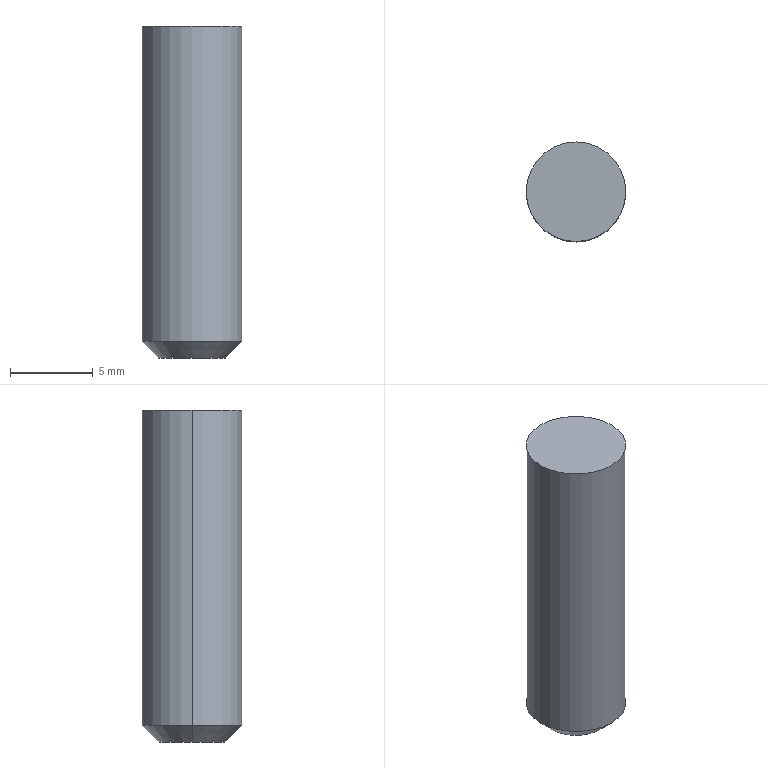Part | SolidWorks | features BaseBody 1 | 1 solid | 6 faces | box 6 x 6 x 20 mm | volume 557.109 mm3 | cylinder 2 | cone 2 | plane 2 | commonest cylinder face diameters 6 x2
STEP:
#1=CARTESIAN_POINT('',(403.071,348.177,19.477));
#2=VERTEX_POINT('',#1);
#3=CARTESIAN_POINT('',(409.071,348.177,19.477));
#4=VERTEX_POINT('',#3);
#5=CARTESIAN_POINT('',(406.071,348.177,19.477));
#6=DIRECTION('',(0.,0.,-1.));
#7=DIRECTION('',(-1.,0.,0.));
#8=AXIS2_PLACEMENT_3D('',#5,#6,#7);
#9=CIRCLE('',#8,3.);
#10=EDGE_CURVE('',#2,#4,#9,.T.);
#11=ORIENTED_EDGE('',*,*,#10,.F.);
#12=CARTESIAN_POINT('',(403.071,348.177,38.477));
#13=VERTEX_POINT('',#12);
#14=CARTESIAN_POINT('',(403.071,348.177,18.477));
#15=DIRECTION('',(0.,0.,1.));
#16=VECTOR('',#15,1000.);
#17=LINE('',#14,#16);
#18=EDGE_CURVE('',#2,#13,#17,.T.);
#19=ORIENTED_EDGE('',*,*,#18,.T.);
#20=CARTESIAN_POINT('',(409.071,348.177,38.477));
#21=VERTEX_POINT('',#20);
#22=CARTESIAN_POINT('',(406.071,348.177,38.477));
#23=DIRECTION('',(0.,0.,1.));
#24=DIRECTION('',(-1.,0.,0.));
#25=AXIS2_PLACEMENT_3D('',#22,#23,#24);
#26=CIRCLE('',#25,3.);
#27=EDGE_CURVE('',#21,#13,#26,.T.);
#28=ORIENTED_EDGE('',*,*,#27,.F.);
#29=CARTESIAN_POINT('',(409.071,348.177,18.477));
#30=DIRECTION('',(0.,0.,1.));
#31=VECTOR('',#30,1000.);
#32=LINE('',#29,#31);
#33=EDGE_CURVE('',#4,#21,#32,.T.);
#34=ORIENTED_EDGE('',*,*,#33,.F.);
#35=EDGE_LOOP('',(#11,#19,#28,#34));
#36=FACE_OUTER_BOUND('',#35,.T.);
#37=CARTESIAN_POINT('',(406.071,348.177,18.477));
#38=DIRECTION('',(0.,0.,1.));
#39=DIRECTION('',(1.,0.,0.));
#40=AXIS2_PLACEMENT_3D('',#37,#38,#39);
#41=CYLINDRICAL_SURFACE('',#40,3.);
#42=ADVANCED_FACE('',(#36),#41,.T.);
#43=CARTESIAN_POINT('',(404.071,348.177,18.477));
#44=VERTEX_POINT('',#43);
#45=CARTESIAN_POINT('',(408.071,348.177,18.477));
#46=VERTEX_POINT('',#45);
#47=CARTESIAN_POINT('',(406.071,348.177,18.477));
#48=DIRECTION('',(0.,0.,-1.));
#49=DIRECTION('',(-1.,0.,0.));
#50=AXIS2_PLACEMENT_3D('',#47,#48,#49);
#51=CIRCLE('',#50,2.);
#52=EDGE_CURVE('',#44,#46,#51,.T.);
#53=ORIENTED_EDGE('',*,*,#52,.F.);
#54=CARTESIAN_POINT('',(403.571,348.177,18.977));
#55=DIRECTION('',(-0.7071,0.,0.7071));
#56=VECTOR('',#55,1000.);
#57=LINE('',#54,#56);
#58=EDGE_CURVE('',#44,#2,#57,.T.);
#59=ORIENTED_EDGE('',*,*,#58,.T.);
#60=ORIENTED_EDGE('',*,*,#10,.T.);
#61=CARTESIAN_POINT('',(408.571,348.177,18.977));
#62=DIRECTION('',(0.7071,0.,0.7071));
#63=VECTOR('',#62,1000.);
#64=LINE('',#61,#63);
#65=EDGE_CURVE('',#46,#4,#64,.T.);
#66=ORIENTED_EDGE('',*,*,#65,.F.);
#67=EDGE_LOOP('',(#53,#59,#60,#66));
#68=FACE_OUTER_BOUND('',#67,.T.);
#69=CARTESIAN_POINT('',(406.071,348.177,18.977));
#70=DIRECTION('',(0.,0.,1.));
#71=DIRECTION('',(1.,0.,0.));
#72=AXIS2_PLACEMENT_3D('',#69,#70,#71);
#73=CONICAL_SURFACE('',#72,2.5,0.7854);
#74=ADVANCED_FACE('',(#68),#73,.T.);
#75=CARTESIAN_POINT('',(406.071,348.177,18.477));
#76=DIRECTION('',(0.,0.,-1.));
#77=DIRECTION('',(-1.,0.,0.));
#78=AXIS2_PLACEMENT_3D('',#75,#76,#77);
#79=CIRCLE('',#78,2.);
#80=EDGE_CURVE('',#46,#44,#79,.T.);
#81=ORIENTED_EDGE('',*,*,#80,.T.);
#82=ORIENTED_EDGE('',*,*,#52,.T.);
#83=EDGE_LOOP('',(#81,#82));
#84=FACE_OUTER_BOUND('',#83,.T.);
#85=CARTESIAN_POINT('',(406.071,348.177,18.477));
#86=DIRECTION('',(0.,0.,-1.));
#87=DIRECTION('',(0.,-1.,0.));
#88=AXIS2_PLACEMENT_3D('',#85,#86,#87);
#89=PLANE('',#88);
#90=ADVANCED_FACE('',(#84),#89,.T.);
#91=ORIENTED_EDGE('',*,*,#58,.F.);
#92=ORIENTED_EDGE('',*,*,#80,.F.);
#93=ORIENTED_EDGE('',*,*,#65,.T.);
#94=CARTESIAN_POINT('',(406.071,348.177,19.477));
#95=DIRECTION('',(0.,0.,-1.));
#96=DIRECTION('',(-1.,0.,0.));
#97=AXIS2_PLACEMENT_3D('',#94,#95,#96);
#98=CIRCLE('',#97,3.);
#99=EDGE_CURVE('',#4,#2,#98,.T.);
#100=ORIENTED_EDGE('',*,*,#99,.T.);
#101=EDGE_LOOP('',(#91,#92,#93,#100));
#102=FACE_OUTER_BOUND('',#101,.T.);
#103=CARTESIAN_POINT('',(406.071,348.177,18.977));
#104=DIRECTION('',(0.,0.,1.));
#105=DIRECTION('',(1.,0.,0.));
#106=AXIS2_PLACEMENT_3D('',#103,#104,#105);
#107=CONICAL_SURFACE('',#106,2.5,0.7854);
#108=ADVANCED_FACE('',(#102),#107,.T.);
#109=ORIENTED_EDGE('',*,*,#18,.F.);
#110=ORIENTED_EDGE('',*,*,#99,.F.);
#111=ORIENTED_EDGE('',*,*,#33,.T.);
#112=CARTESIAN_POINT('',(406.071,348.177,38.477));
#113=DIRECTION('',(0.,0.,1.));
#114=DIRECTION('',(-1.,0.,0.));
#115=AXIS2_PLACEMENT_3D('',#112,#113,#114);
#116=CIRCLE('',#115,3.);
#117=EDGE_CURVE('',#13,#21,#116,.T.);
#118=ORIENTED_EDGE('',*,*,#117,.F.);
#119=EDGE_LOOP('',(#109,#110,#111,#118));
#120=FACE_OUTER_BOUND('',#119,.T.);
#121=CARTESIAN_POINT('',(406.071,348.177,18.477));
#122=DIRECTION('',(0.,0.,1.));
#123=DIRECTION('',(1.,0.,0.));
#124=AXIS2_PLACEMENT_3D('',#121,#122,#123);
#125=CYLINDRICAL_SURFACE('',#124,3.);
#126=ADVANCED_FACE('',(#120),#125,.T.);
#127=ORIENTED_EDGE('',*,*,#27,.T.);
#128=ORIENTED_EDGE('',*,*,#117,.T.);
#129=EDGE_LOOP('',(#127,#128));
#130=FACE_OUTER_BOUND('',#129,.T.);
#131=CARTESIAN_POINT('',(406.071,348.177,38.477));
#132=DIRECTION('',(0.,0.,1.));
#133=DIRECTION('',(1.,0.,0.));
#134=AXIS2_PLACEMENT_3D('',#131,#132,#133);
#135=PLANE('',#134);
#136=ADVANCED_FACE('',(#130),#135,.T.);
#137=CLOSED_SHELL('',(#42,#74,#90,#108,#126,#136));
#138=MANIFOLD_SOLID_BREP('',#137);
#139=CARTESIAN_POINT('',(0.,0.,0.));
#140=DIRECTION('',(0.,0.,1.));
#141=DIRECTION('',(1.,0.,0.));
#142=AXIS2_PLACEMENT_3D('',#139,#140,#141);
#143=(LENGTH_UNIT()NAMED_UNIT(*)SI_UNIT(.MILLI.,.METRE.));
#144=UNCERTAINTY_MEASURE_WITH_UNIT(LENGTH_MEASURE(0.00001),#143,'','');
#145=(NAMED_UNIT(*)PLANE_ANGLE_UNIT()SI_UNIT($,.RADIAN.));
#146=(NAMED_UNIT(*)SI_UNIT($,.STERADIAN.)SOLID_ANGLE_UNIT());
#147=(GEOMETRIC_REPRESENTATION_CONTEXT(3)GLOBAL_UNCERTAINTY_ASSIGNED_CONTEXT((#144))GLOBAL_UNIT_ASSIGNED_CONTEXT((#143,#145,#146))REPRESENTATION_CONTEXT('',''));
#148=ADVANCED_BREP_SHAPE_REPRESENTATION('',(#138,#142),#147);